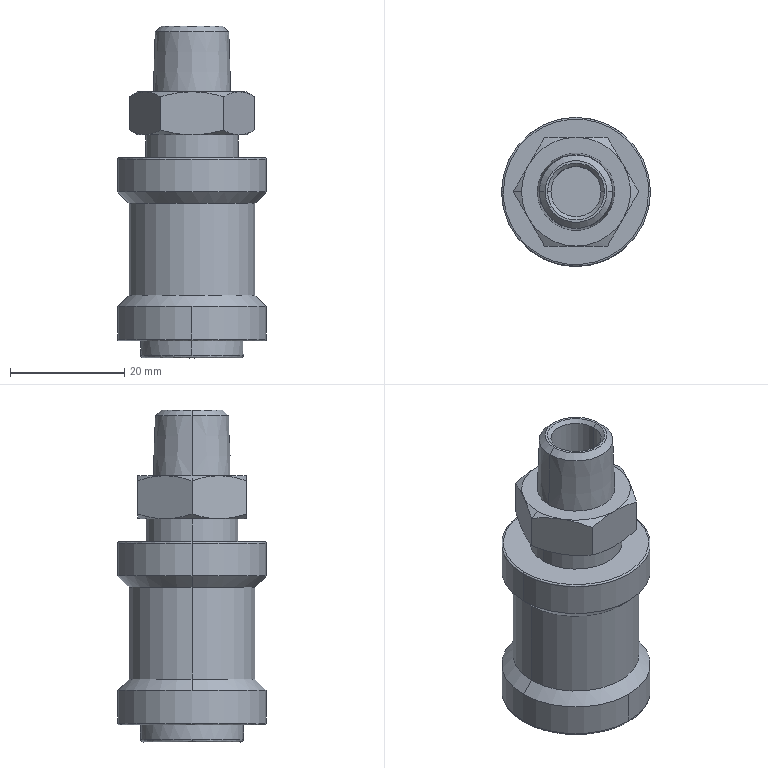Part | STEP file | 1 solid | 58 faces | box 26 x 26 x 58 mm | volume 16455 mm3 | cone 26 | plane 14 | cylinder 12 | spline 6 | commonest cylinder face diameters 26 x4 8.771 x2 16.078 x2 18 x2 22 x2